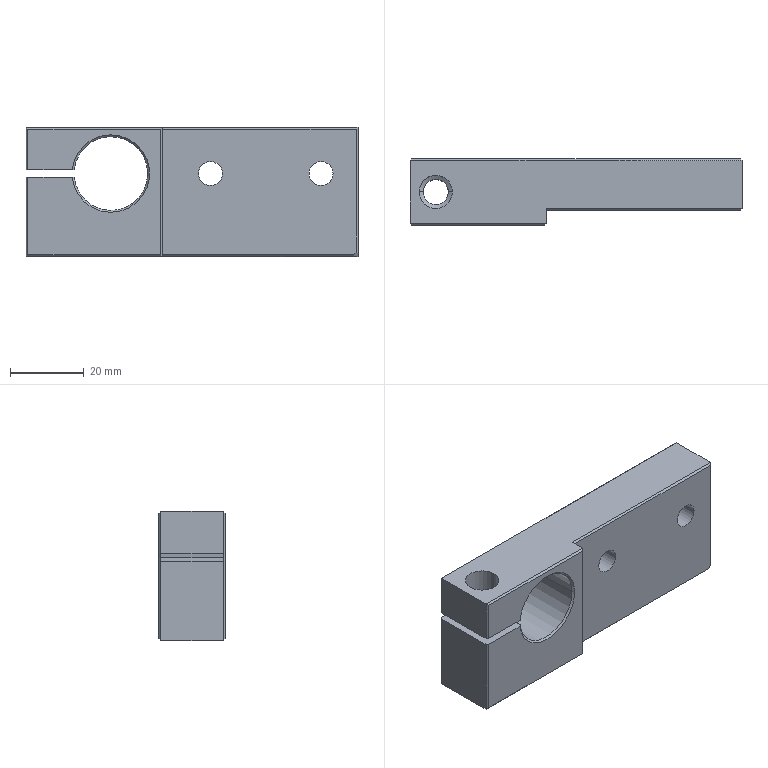Part | NX | 1 solid | 46 faces | box 90 x 18 x 35 mm | volume 39820 mm3 | plane 27 | cylinder 14 | cone 5 | commonest cylinder face diameters 6.5 x4 11 x4 6.8 x2 9 x2 20 x2
STEP:
#1=CARTESIAN_POINT('',(0.5,18.,-17.));
#2=VERTEX_POINT('',#1);
#3=CARTESIAN_POINT('',(0.,17.5,-17.5));
#4=VERTEX_POINT('',#3);
#5=CARTESIAN_POINT('',(17.5,35.,0.));
#6=DIRECTION('',(-0.5774,-0.5774,-0.5774));
#7=VECTOR('',#6,1000.);
#8=LINE('',#5,#7);
#9=EDGE_CURVE('',#2,#4,#8,.T.);
#10=ORIENTED_EDGE('',*,*,#9,.T.);
#11=CARTESIAN_POINT('',(0.,17.5,4.));
#12=VERTEX_POINT('',#11);
#13=CARTESIAN_POINT('',(0.,17.5,0.));
#14=DIRECTION('',(0.,0.,1.));
#15=VECTOR('',#14,1000.);
#16=LINE('',#13,#15);
#17=EDGE_CURVE('',#4,#12,#16,.T.);
#18=ORIENTED_EDGE('',*,*,#17,.T.);
#19=CARTESIAN_POINT('',(0.5,18.,4.));
#20=VERTEX_POINT('',#19);
#21=CARTESIAN_POINT('',(-17.5,0.,4.));
#22=DIRECTION('',(0.7071,0.7071,0.));
#23=VECTOR('',#22,1000.);
#24=LINE('',#21,#23);
#25=EDGE_CURVE('',#12,#20,#24,.T.);
#26=ORIENTED_EDGE('',*,*,#25,.T.);
#27=CARTESIAN_POINT('',(0.5,18.,0.));
#28=DIRECTION('',(0.,0.,1.));
#29=VECTOR('',#28,1000.);
#30=LINE('',#27,#29);
#31=EDGE_CURVE('',#2,#20,#30,.T.);
#32=ORIENTED_EDGE('',*,*,#31,.F.);
#33=EDGE_LOOP('',(#10,#18,#26,#32));
#34=FACE_BOUND('',#33,.T.);
#35=CARTESIAN_POINT('',(0.,17.5,-16.5));
#36=DIRECTION('',(-0.7071,0.7071,0.));
#37=DIRECTION('',(0.,0.,1.));
#38=AXIS2_PLACEMENT_3D('',#35,#36,#37);
#39=PLANE('',#38);
#40=ADVANCED_FACE('',(#34),#39,.T.);
#41=CARTESIAN_POINT('',(37.,0.5,-17.5));
#42=VERTEX_POINT('',#41);
#43=CARTESIAN_POINT('',(36.5,0.,-17.));
#44=VERTEX_POINT('',#43);
#45=CARTESIAN_POINT('',(19.5,-17.,0.));
#46=DIRECTION('',(-0.5774,-0.5774,0.5774));
#47=VECTOR('',#46,1000.);
#48=LINE('',#45,#47);
#49=EDGE_CURVE('',#42,#44,#48,.T.);
#50=ORIENTED_EDGE('',*,*,#49,.T.);
#51=CARTESIAN_POINT('',(0.5,0.,-17.));
#52=VERTEX_POINT('',#51);
#53=CARTESIAN_POINT('',(0.,0.,-17.));
#54=DIRECTION('',(1.,0.,0.));
#55=VECTOR('',#54,1000.);
#56=LINE('',#53,#55);
#57=EDGE_CURVE('',#52,#44,#56,.T.);
#58=ORIENTED_EDGE('',*,*,#57,.F.);
#59=CARTESIAN_POINT('',(0.,0.5,-17.5));
#60=VERTEX_POINT('',#59);
#61=CARTESIAN_POINT('',(17.5,-17.,0.));
#62=DIRECTION('',(0.5774,-0.5774,0.5774));
#63=VECTOR('',#62,1000.);
#64=LINE('',#61,#63);
#65=EDGE_CURVE('',#60,#52,#64,.T.);
#66=ORIENTED_EDGE('',*,*,#65,.F.);
#67=CARTESIAN_POINT('',(0.,0.5,-17.5));
#68=DIRECTION('',(-1.,0.,0.));
#69=VECTOR('',#68,1000.);
#70=LINE('',#67,#69);
#71=EDGE_CURVE('',#42,#60,#70,.T.);
#72=ORIENTED_EDGE('',*,*,#71,.F.);
#73=EDGE_LOOP('',(#50,#58,#66,#72));
#74=FACE_BOUND('',#73,.T.);
#75=CARTESIAN_POINT('',(1.,0.5,-17.5));
#76=DIRECTION('',(0.,-0.7071,-0.7071));
#77=DIRECTION('',(0.,-0.7071,0.7071));
#78=AXIS2_PLACEMENT_3D('',#75,#76,#77);
#79=PLANE('',#78);
#80=ADVANCED_FACE('',(#74),#79,.T.);
#81=CARTESIAN_POINT('',(37.,4.,17.));
#82=VERTEX_POINT('',#81);
#83=CARTESIAN_POINT('',(37.,4.,-17.));
#84=VERTEX_POINT('',#83);
#85=CARTESIAN_POINT('',(37.,4.,0.));
#86=DIRECTION('',(0.,0.,-1.));
#87=VECTOR('',#86,1000.);
#88=LINE('',#85,#87);
#89=EDGE_CURVE('',#82,#84,#88,.T.);
#90=ORIENTED_EDGE('',*,*,#89,.F.);
#91=CARTESIAN_POINT('',(37.,4.5,17.5));
#92=VERTEX_POINT('',#91);
#93=CARTESIAN_POINT('',(37.,-13.,0.));
#94=DIRECTION('',(0.,-0.7071,-0.7071));
#95=VECTOR('',#94,1000.);
#96=LINE('',#93,#95);
#97=EDGE_CURVE('',#92,#82,#96,.T.);
#98=ORIENTED_EDGE('',*,*,#97,.F.);
#99=CARTESIAN_POINT('',(37.,0.5,17.5));
#100=VERTEX_POINT('',#99);
#101=CARTESIAN_POINT('',(37.,0.,17.5));
#102=DIRECTION('',(0.,-1.,0.));
#103=VECTOR('',#102,1000.);
#104=LINE('',#101,#103);
#105=EDGE_CURVE('',#92,#100,#104,.T.);
#106=ORIENTED_EDGE('',*,*,#105,.T.);
#107=CARTESIAN_POINT('',(37.,0.5,0.));
#108=DIRECTION('',(0.,0.,-1.));
#109=VECTOR('',#108,1000.);
#110=LINE('',#107,#109);
#111=EDGE_CURVE('',#100,#42,#110,.T.);
#112=ORIENTED_EDGE('',*,*,#111,.T.);
#113=CARTESIAN_POINT('',(37.,4.5,-17.5));
#114=VERTEX_POINT('',#113);
#115=CARTESIAN_POINT('',(37.,0.,-17.5));
#116=DIRECTION('',(0.,1.,0.));
#117=VECTOR('',#116,1000.);
#118=LINE('',#115,#117);
#119=EDGE_CURVE('',#42,#114,#118,.T.);
#120=ORIENTED_EDGE('',*,*,#119,.T.);
#121=CARTESIAN_POINT('',(37.,-13.,0.));
#122=DIRECTION('',(0.,0.7071,-0.7071));
#123=VECTOR('',#122,1000.);
#124=LINE('',#121,#123);
#125=EDGE_CURVE('',#84,#114,#124,.T.);
#126=ORIENTED_EDGE('',*,*,#125,.F.);
#127=EDGE_LOOP('',(#90,#98,#106,#112,#120,#126));
#128=FACE_BOUND('',#127,.T.);
#129=CARTESIAN_POINT('',(37.,0.,-17.5));
#130=DIRECTION('',(1.,0.,0.));
#131=DIRECTION('',(0.,1.,0.));
#132=AXIS2_PLACEMENT_3D('',#129,#130,#131);
#133=PLANE('',#132);
#134=ADVANCED_FACE('',(#128),#133,.T.);
#135=CARTESIAN_POINT('',(44.5,11.5,5.));
#136=VERTEX_POINT('',#135);
#137=CARTESIAN_POINT('',(55.5,11.5,5.));
#138=VERTEX_POINT('',#137);
#139=CARTESIAN_POINT('',(50.,11.5,5.));
#140=DIRECTION('',(0.,1.,0.));
#141=DIRECTION('',(1.,0.,0.));
#142=AXIS2_PLACEMENT_3D('',#139,#140,#141);
#143=CIRCLE('',#142,5.5);
#144=EDGE_CURVE('',#136,#138,#143,.T.);
#145=ORIENTED_EDGE('',*,*,#144,.T.);
#146=CARTESIAN_POINT('',(50.,11.5,5.));
#147=DIRECTION('',(0.,1.,0.));
#148=DIRECTION('',(1.,0.,0.));
#149=AXIS2_PLACEMENT_3D('',#146,#147,#148);
#150=CIRCLE('',#149,5.5);
#151=EDGE_CURVE('',#138,#136,#150,.T.);
#152=ORIENTED_EDGE('',*,*,#151,.T.);
#153=EDGE_LOOP('',(#145,#152));
#154=FACE_BOUND('',#153,.T.);
#155=CARTESIAN_POINT('',(53.25,11.5,5.));
#156=VERTEX_POINT('',#155);
#157=CARTESIAN_POINT('',(46.75,11.5,5.));
#158=VERTEX_POINT('',#157);
#159=CARTESIAN_POINT('',(50.,11.5,5.));
#160=DIRECTION('',(0.,1.,0.));
#161=DIRECTION('',(1.,0.,0.));
#162=AXIS2_PLACEMENT_3D('',#159,#160,#161);
#163=CIRCLE('',#162,3.25);
#164=EDGE_CURVE('',#156,#158,#163,.T.);
#165=ORIENTED_EDGE('',*,*,#164,.F.);
#166=CARTESIAN_POINT('',(50.,11.5,5.));
#167=DIRECTION('',(0.,1.,0.));
#168=DIRECTION('',(1.,0.,0.));
#169=AXIS2_PLACEMENT_3D('',#166,#167,#168);
#170=CIRCLE('',#169,3.25);
#171=EDGE_CURVE('',#158,#156,#170,.T.);
#172=ORIENTED_EDGE('',*,*,#171,.F.);
#173=EDGE_LOOP('',(#165,#172));
#174=FACE_BOUND('',#173,.T.);
#175=CARTESIAN_POINT('',(50.,11.5,5.));
#176=DIRECTION('',(0.,1.,0.));
#177=DIRECTION('',(1.,0.,0.));
#178=AXIS2_PLACEMENT_3D('',#175,#176,#177);
#179=PLANE('',#178);
#180=ADVANCED_FACE('',(#154,#174),#179,.T.);
#181=CARTESIAN_POINT('',(74.5,11.5,5.));
#182=VERTEX_POINT('',#181);
#183=CARTESIAN_POINT('',(85.5,11.5,5.));
#184=VERTEX_POINT('',#183);
#185=CARTESIAN_POINT('',(80.,11.5,5.));
#186=DIRECTION('',(0.,1.,0.));
#187=DIRECTION('',(1.,0.,0.));
#188=AXIS2_PLACEMENT_3D('',#185,#186,#187);
#189=CIRCLE('',#188,5.5);
#190=EDGE_CURVE('',#182,#184,#189,.T.);
#191=ORIENTED_EDGE('',*,*,#190,.F.);
#192=CARTESIAN_POINT('',(74.5,18.,5.));
#193=VERTEX_POINT('',#192);
#194=CARTESIAN_POINT('',(74.5,-2.79,5.));
#195=DIRECTION('',(0.,1.,0.));
#196=VECTOR('',#195,1000.);
#197=LINE('',#194,#196);
#198=EDGE_CURVE('',#182,#193,#197,.T.);
#199=ORIENTED_EDGE('',*,*,#198,.T.);
#200=CARTESIAN_POINT('',(85.5,18.,5.));
#201=VERTEX_POINT('',#200);
#202=CARTESIAN_POINT('',(80.,18.,5.));
#203=DIRECTION('',(0.,1.,0.));
#204=DIRECTION('',(1.,0.,0.));
#205=AXIS2_PLACEMENT_3D('',#202,#203,#204);
#206=CIRCLE('',#205,5.5);
#207=EDGE_CURVE('',#193,#201,#206,.T.);
#208=ORIENTED_EDGE('',*,*,#207,.T.);
#209=CARTESIAN_POINT('',(85.5,-2.79,5.));
#210=DIRECTION('',(0.,1.,0.));
#211=VECTOR('',#210,1000.);
#212=LINE('',#209,#211);
#213=EDGE_CURVE('',#184,#201,#212,.T.);
#214=ORIENTED_EDGE('',*,*,#213,.F.);
#215=EDGE_LOOP('',(#191,#199,#208,#214));
#216=FACE_BOUND('',#215,.T.);
#217=CARTESIAN_POINT('',(80.,-2.79,5.));
#218=DIRECTION('',(0.,1.,0.));
#219=DIRECTION('',(1.,0.,0.));
#220=AXIS2_PLACEMENT_3D('',#217,#218,#219);
#221=CYLINDRICAL_SURFACE('',#220,5.5);
#222=ADVANCED_FACE('',(#216),#221,.F.);
#223=CARTESIAN_POINT('',(90.,17.5,17.5));
#224=VERTEX_POINT('',#223);
#225=CARTESIAN_POINT('',(89.5,18.,17.));
#226=VERTEX_POINT('',#225);
#227=CARTESIAN_POINT('',(72.5,35.,0.));
#228=DIRECTION('',(-0.5774,0.5774,-0.5774));
#229=VECTOR('',#228,1000.);
#230=LINE('',#227,#229);
#231=EDGE_CURVE('',#224,#226,#230,.T.);
#232=ORIENTED_EDGE('',*,*,#231,.F.);
#233=CARTESIAN_POINT('',(90.,17.5,-17.5));
#234=VERTEX_POINT('',#233);
#235=CARTESIAN_POINT('',(90.,17.5,0.));
#236=DIRECTION('',(0.,0.,-1.));
#237=VECTOR('',#236,1000.);
#238=LINE('',#235,#237);
#239=EDGE_CURVE('',#224,#234,#238,.T.);
#240=ORIENTED_EDGE('',*,*,#239,.T.);
#241=CARTESIAN_POINT('',(89.5,18.,-17.));
#242=VERTEX_POINT('',#241);
#243=CARTESIAN_POINT('',(72.5,35.,0.));
#244=DIRECTION('',(-0.5774,0.5774,0.5774));
#245=VECTOR('',#244,1000.);
#246=LINE('',#243,#245);
#247=EDGE_CURVE('',#234,#242,#246,.T.);
#248=ORIENTED_EDGE('',*,*,#247,.T.);
#249=CARTESIAN_POINT('',(89.5,18.,0.));
#250=DIRECTION('',(0.,0.,1.));
#251=VECTOR('',#250,1000.);
#252=LINE('',#249,#251);
#253=EDGE_CURVE('',#242,#226,#252,.T.);
#254=ORIENTED_EDGE('',*,*,#253,.T.);
#255=EDGE_LOOP('',(#232,#240,#248,#254));
#256=FACE_BOUND('',#255,.T.);
#257=CARTESIAN_POINT('',(89.5,18.,-16.5));
#258=DIRECTION('',(0.7071,0.7071,0.));
#259=DIRECTION('',(0.,0.,-1.));
#260=AXIS2_PLACEMENT_3D('',#257,#258,#259);
#261=PLANE('',#260);
#262=ADVANCED_FACE('',(#256),#261,.T.);
#263=CARTESIAN_POINT('',(10.4,9.,-17.5));
#264=VERTEX_POINT('',#263);
#265=CARTESIAN_POINT('',(3.6,9.,-17.5));
#266=VERTEX_POINT('',#265);
#267=CARTESIAN_POINT('',(7.,9.,-17.5));
#268=DIRECTION('',(0.,0.,1.));
#269=DIRECTION('',(1.,0.,0.));
#270=AXIS2_PLACEMENT_3D('',#267,#268,#269);
#271=CIRCLE('',#270,3.4);
#272=EDGE_CURVE('',#264,#266,#271,.T.);
#273=ORIENTED_EDGE('',*,*,#272,.F.);
#274=CARTESIAN_POINT('',(10.4,9.,3.329));
#275=VERTEX_POINT('',#274);
#276=CARTESIAN_POINT('',(10.4,9.,4.));
#277=DIRECTION('',(0.,0.,1.));
#278=VECTOR('',#277,1000.);
#279=LINE('',#276,#278);
#280=EDGE_CURVE('',#264,#275,#279,.T.);
#281=ORIENTED_EDGE('',*,*,#280,.T.);
#282=CARTESIAN_POINT('',(3.6,9.,3.329));
#283=VERTEX_POINT('',#282);
#284=CARTESIAN_POINT('',(7.,9.,3.329));
#285=DIRECTION('',(0.,0.,1.));
#286=DIRECTION('',(1.,0.,0.));
#287=AXIS2_PLACEMENT_3D('',#284,#285,#286);
#288=CIRCLE('',#287,3.4);
#289=EDGE_CURVE('',#275,#283,#288,.T.);
#290=ORIENTED_EDGE('',*,*,#289,.T.);
#291=CARTESIAN_POINT('',(3.6,9.,4.));
#292=DIRECTION('',(0.,0.,1.));
#293=VECTOR('',#292,1000.);
#294=LINE('',#291,#293);
#295=EDGE_CURVE('',#266,#283,#294,.T.);
#296=ORIENTED_EDGE('',*,*,#295,.F.);
#297=EDGE_LOOP('',(#273,#281,#290,#296));
#298=FACE_BOUND('',#297,.T.);
#299=CARTESIAN_POINT('',(7.,9.,4.));
#300=DIRECTION('',(0.,0.,1.));
#301=DIRECTION('',(1.,0.,0.));
#302=AXIS2_PLACEMENT_3D('',#299,#300,#301);
#303=CYLINDRICAL_SURFACE('',#302,3.4);
#304=ADVANCED_FACE('',(#298),#303,.F.);
#305=CARTESIAN_POINT('',(76.75,4.,5.));
#306=VERTEX_POINT('',#305);
#307=CARTESIAN_POINT('',(83.25,4.,5.));
#308=VERTEX_POINT('',#307);
#309=CARTESIAN_POINT('',(80.,4.,5.));
#310=DIRECTION('',(0.,1.,0.));
#311=DIRECTION('',(1.,0.,0.));
#312=AXIS2_PLACEMENT_3D('',#309,#310,#311);
#313=CIRCLE('',#312,3.25);
#314=EDGE_CURVE('',#306,#308,#313,.T.);
#315=ORIENTED_EDGE('',*,*,#314,.F.);
#316=CARTESIAN_POINT('',(76.75,11.5,5.));
#317=VERTEX_POINT('',#316);
#318=CARTESIAN_POINT('',(76.75,-2.79,5.));
#319=DIRECTION('',(0.,1.,0.));
#320=VECTOR('',#319,1000.);
#321=LINE('',#318,#320);
#322=EDGE_CURVE('',#306,#317,#321,.T.);
#323=ORIENTED_EDGE('',*,*,#322,.T.);
#324=CARTESIAN_POINT('',(83.25,11.5,5.));
#325=VERTEX_POINT('',#324);
#326=CARTESIAN_POINT('',(80.,11.5,5.));
#327=DIRECTION('',(0.,1.,0.));
#328=DIRECTION('',(1.,0.,0.));
#329=AXIS2_PLACEMENT_3D('',#326,#327,#328);
#330=CIRCLE('',#329,3.25);
#331=EDGE_CURVE('',#317,#325,#330,.T.);
#332=ORIENTED_EDGE('',*,*,#331,.T.);
#333=CARTESIAN_POINT('',(83.25,-2.79,5.));
#334=DIRECTION('',(0.,1.,0.));
#335=VECTOR('',#334,1000.);
#336=LINE('',#333,#335);
#337=EDGE_CURVE('',#308,#325,#336,.T.);
#338=ORIENTED_EDGE('',*,*,#337,.F.);
#339=EDGE_LOOP('',(#315,#323,#332,#338));
#340=FACE_BOUND('',#339,.T.);
#341=CARTESIAN_POINT('',(80.,-2.79,5.));
#342=DIRECTION('',(0.,1.,0.));
#343=DIRECTION('',(1.,0.,0.));
#344=AXIS2_PLACEMENT_3D('',#341,#342,#343);
#345=CYLINDRICAL_SURFACE('',#344,3.25);
#346=ADVANCED_FACE('',(#340),#345,.F.);
#347=CARTESIAN_POINT('',(90.,5.207,-17.5));
#348=VERTEX_POINT('',#347);
#349=CARTESIAN_POINT('',(90.,4.5,-16.5));
#350=VERTEX_POINT('',#349);
#351=CARTESIAN_POINT('',(90.,-7.167,0.));
#352=DIRECTION('',(0.,-0.5774,0.8165));
#353=VECTOR('',#352,1000.);
#354=LINE('',#351,#353);
#355=EDGE_CURVE('',#348,#350,#354,.T.);
#356=ORIENTED_EDGE('',*,*,#355,.T.);
#357=CARTESIAN_POINT('',(89.5,4.,-16.293));
#358=VERTEX_POINT('',#357);
#359=CARTESIAN_POINT('',(0.,-85.5,20.779));
#360=DIRECTION('',(-0.6786,-0.6786,0.2811));
#361=VECTOR('',#360,1000.);
#362=LINE('',#359,#361);
#363=EDGE_CURVE('',#350,#358,#362,.T.);
#364=ORIENTED_EDGE('',*,*,#363,.T.);
#365=CARTESIAN_POINT('',(88.793,4.,-17.));
#366=VERTEX_POINT('',#365);
#367=CARTESIAN_POINT('',(105.793,4.,0.));
#368=DIRECTION('',(-0.7071,0.,-0.7071));
#369=VECTOR('',#368,1000.);
#370=LINE('',#367,#369);
#371=EDGE_CURVE('',#358,#366,#370,.T.);
#372=ORIENTED_EDGE('',*,*,#371,.T.);
#373=CARTESIAN_POINT('',(89.,4.5,-17.5));
#374=VERTEX_POINT('',#373);
#375=CARTESIAN_POINT('',(81.751,-13.,0.));
#376=DIRECTION('',(0.2811,0.6786,-0.6786));
#377=VECTOR('',#376,1000.);
#378=LINE('',#375,#377);
#379=EDGE_CURVE('',#366,#374,#378,.T.);
#380=ORIENTED_EDGE('',*,*,#379,.T.);
#381=CARTESIAN_POINT('',(0.,-58.433,-17.5));
#382=DIRECTION('',(-0.8165,-0.5774,0.));
#383=VECTOR('',#382,1000.);
#384=LINE('',#381,#383);
#385=EDGE_CURVE('',#348,#374,#384,.T.);
#386=ORIENTED_EDGE('',*,*,#385,.F.);
#387=EDGE_LOOP('',(#356,#364,#372,#380,#386));
#388=FACE_BOUND('',#387,.T.);
#389=CARTESIAN_POINT('',(89.,4.5,-17.5));
#390=DIRECTION('',(0.5,-0.7071,-0.5));
#391=DIRECTION('',(0.,0.5774,-0.8165));
#392=AXIS2_PLACEMENT_3D('',#389,#390,#391);
#393=PLANE('',#392);
#394=ADVANCED_FACE('',(#388),#393,.T.);
#395=CARTESIAN_POINT('',(0.,4.5,-17.5));
#396=DIRECTION('',(1.,0.,0.));
#397=VECTOR('',#396,1000.);
#398=LINE('',#395,#397);
#399=EDGE_CURVE('',#114,#374,#398,.T.);
#400=ORIENTED_EDGE('',*,*,#399,.T.);
#401=ORIENTED_EDGE('',*,*,#379,.F.);
#402=CARTESIAN_POINT('',(0.,4.,-17.));
#403=DIRECTION('',(-1.,0.,0.));
#404=VECTOR('',#403,1000.);
#405=LINE('',#402,#404);
#406=EDGE_CURVE('',#366,#84,#405,.T.);
#407=ORIENTED_EDGE('',*,*,#406,.T.);
#408=ORIENTED_EDGE('',*,*,#125,.T.);
#409=EDGE_LOOP('',(#400,#401,#407,#408));
#410=FACE_BOUND('',#409,.T.);
#411=CARTESIAN_POINT('',(37.,4.5,-17.5));
#412=DIRECTION('',(0.,-0.7071,-0.7071));
#413=DIRECTION('',(0.,-0.7071,0.7071));
#414=AXIS2_PLACEMENT_3D('',#411,#412,#413);
#415=PLANE('',#414);
#416=ADVANCED_FACE('',(#410),#415,.T.);
#417=CARTESIAN_POINT('',(0.,0.5,17.5));
#418=VERTEX_POINT('',#417);
#419=CARTESIAN_POINT('',(0.5,0.,17.));
#420=VERTEX_POINT('',#419);
#421=CARTESIAN_POINT('',(17.5,-17.,0.));
#422=DIRECTION('',(0.5774,-0.5774,-0.5774));
#423=VECTOR('',#422,1000.);
#424=LINE('',#421,#423);
#425=EDGE_CURVE('',#418,#420,#424,.T.);
#426=ORIENTED_EDGE('',*,*,#425,.F.);
#427=CARTESIAN_POINT('',(0.,0.5,6.));
#428=VERTEX_POINT('',#427);
#429=CARTESIAN_POINT('',(0.,0.5,0.));
#430=DIRECTION('',(0.,0.,1.));
#431=VECTOR('',#430,1000.);
#432=LINE('',#429,#431);
#433=EDGE_CURVE('',#428,#418,#432,.T.);
#434=ORIENTED_EDGE('',*,*,#433,.F.);
#435=CARTESIAN_POINT('',(0.5,0.,6.));
#436=VERTEX_POINT('',#435);
#437=CARTESIAN_POINT('',(0.5,0.,6.));
#438=DIRECTION('',(0.7071,-0.7071,0.));
#439=VECTOR('',#438,1000.);
#440=LINE('',#437,#439);
#441=EDGE_CURVE('',#428,#436,#440,.T.);
#442=ORIENTED_EDGE('',*,*,#441,.T.);
#443=CARTESIAN_POINT('',(0.5,0.,0.));
#444=DIRECTION('',(0.,0.,-1.));
#445=VECTOR('',#444,1000.);
#446=LINE('',#443,#445);
#447=EDGE_CURVE('',#420,#436,#446,.T.);
#448=ORIENTED_EDGE('',*,*,#447,.F.);
#449=EDGE_LOOP('',(#426,#434,#442,#448));
#450=FACE_BOUND('',#449,.T.);
#451=CARTESIAN_POINT('',(0.5,0.,6.));
#452=DIRECTION('',(-0.7071,-0.7071,0.));
#453=DIRECTION('',(-0.7071,0.7071,0.));
#454=AXIS2_PLACEMENT_3D('',#451,#452,#453);
#455=PLANE('',#454);
#456=ADVANCED_FACE('',(#450),#455,.T.);
#457=ORIENTED_EDGE('',*,*,#111,.F.);
#458=CARTESIAN_POINT('',(36.5,0.,17.));
#459=VERTEX_POINT('',#458);
#460=CARTESIAN_POINT('',(19.5,-17.,0.));
#461=DIRECTION('',(-0.5774,-0.5774,-0.5774));
#462=VECTOR('',#461,1000.);
#463=LINE('',#460,#462);
#464=EDGE_CURVE('',#100,#459,#463,.T.);
#465=ORIENTED_EDGE('',*,*,#464,.T.);
#466=CARTESIAN_POINT('',(36.5,0.,0.));
#467=DIRECTION('',(0.,0.,1.));
#468=VECTOR('',#467,1000.);
#469=LINE('',#466,#468);
#470=EDGE_CURVE('',#44,#459,#469,.T.);
#471=ORIENTED_EDGE('',*,*,#470,.F.);
#472=ORIENTED_EDGE('',*,*,#49,.F.);
#473=EDGE_LOOP('',(#457,#465,#471,#472));
#474=FACE_BOUND('',#473,.T.);
#475=CARTESIAN_POINT('',(37.,0.5,-17.));
#476=DIRECTION('',(0.7071,-0.7071,0.));
#477=DIRECTION('',(0.,0.,-1.));
#478=AXIS2_PLACEMENT_3D('',#475,#476,#477);
#479=PLANE('',#478);
#480=ADVANCED_FACE('',(#474),#479,.T.);
#481=ORIENTED_EDGE('',*,*,#119,.F.);
#482=ORIENTED_EDGE('',*,*,#71,.T.);
#483=CARTESIAN_POINT('',(0.,0.,-17.5));
#484=DIRECTION('',(0.,1.,0.));
#485=VECTOR('',#484,1000.);
#486=LINE('',#483,#485);
#487=EDGE_CURVE('',#60,#4,#486,.T.);
#488=ORIENTED_EDGE('',*,*,#487,.T.);
#489=CARTESIAN_POINT('',(0.,17.5,-17.5));
#490=DIRECTION('',(1.,0.,0.));
#491=VECTOR('',#490,1000.);
#492=LINE('',#489,#491);
#493=EDGE_CURVE('',#4,#234,#492,.T.);
#494=ORIENTED_EDGE('',*,*,#493,.T.);
#495=CARTESIAN_POINT('',(90.,0.,-17.5));
#496=DIRECTION('',(0.,-1.,0.));
#497=VECTOR('',#496,1000.);
#498=LINE('',#495,#497);
#499=EDGE_CURVE('',#234,#348,#498,.T.);
#500=ORIENTED_EDGE('',*,*,#499,.T.);
#501=ORIENTED_EDGE('',*,*,#385,.T.);
#502=ORIENTED_EDGE('',*,*,#399,.F.);
#503=EDGE_LOOP('',(#481,#482,#488,#494,#500,#501,#502));
#504=FACE_BOUND('',#503,.T.);
#505=ORIENTED_EDGE('',*,*,#272,.T.);
#506=CARTESIAN_POINT('',(7.,9.,-17.5));
#507=DIRECTION('',(0.,0.,1.));
#508=DIRECTION('',(1.,0.,0.));
#509=AXIS2_PLACEMENT_3D('',#506,#507,#508);
#510=CIRCLE('',#509,3.4);
#511=EDGE_CURVE('',#266,#264,#510,.T.);
#512=ORIENTED_EDGE('',*,*,#511,.T.);
#513=EDGE_LOOP('',(#505,#512));
#514=FACE_BOUND('',#513,.T.);
#515=CARTESIAN_POINT('',(0.,0.,-17.5));
#516=DIRECTION('',(0.,0.,1.));
#517=DIRECTION('',(1.,0.,0.));
#518=AXIS2_PLACEMENT_3D('',#515,#516,#517);
#519=PLANE('',#518);
#520=ADVANCED_FACE('',(#504,#514),#519,.F.);
#521=CARTESIAN_POINT('',(90.,4.5,17.5));
#522=VERTEX_POINT('',#521);
#523=CARTESIAN_POINT('',(90.,0.,17.5));
#524=DIRECTION('',(0.,-1.,0.));
#525=VECTOR('',#524,1000.);
#526=LINE('',#523,#525);
#527=EDGE_CURVE('',#224,#522,#526,.T.);
#528=ORIENTED_EDGE('',*,*,#527,.F.);
#529=CARTESIAN_POINT('',(0.,17.5,17.5));
#530=VERTEX_POINT('',#529);
#531=CARTESIAN_POINT('',(0.,17.5,17.5));
#532=DIRECTION('',(-1.,0.,0.));
#533=VECTOR('',#532,1000.);
#534=LINE('',#531,#533);
#535=EDGE_CURVE('',#224,#530,#534,.T.);
#536=ORIENTED_EDGE('',*,*,#535,.T.);
#537=CARTESIAN_POINT('',(0.,0.,17.5));
#538=DIRECTION('',(0.,1.,0.));
#539=VECTOR('',#538,1000.);
#540=LINE('',#537,#539);
#541=EDGE_CURVE('',#418,#530,#540,.T.);
#542=ORIENTED_EDGE('',*,*,#541,.F.);
#543=CARTESIAN_POINT('',(0.,0.5,17.5));
#544=DIRECTION('',(1.,0.,0.));
#545=VECTOR('',#544,1000.);
#546=LINE('',#543,#545);
#547=EDGE_CURVE('',#418,#100,#546,.T.);
#548=ORIENTED_EDGE('',*,*,#547,.T.);
#549=ORIENTED_EDGE('',*,*,#105,.F.);
#550=CARTESIAN_POINT('',(0.,4.5,17.5));
#551=DIRECTION('',(1.,0.,0.));
#552=VECTOR('',#551,1000.);
#553=LINE('',#550,#552);
#554=EDGE_CURVE('',#92,#522,#553,.T.);
#555=ORIENTED_EDGE('',*,*,#554,.T.);
#556=EDGE_LOOP('',(#528,#536,#542,#548,#549,#555));
#557=FACE_BOUND('',#556,.T.);
#558=CARTESIAN_POINT('',(11.5,9.,17.5));
#559=VERTEX_POINT('',#558);
#560=CARTESIAN_POINT('',(2.5,9.,17.5));
#561=VERTEX_POINT('',#560);
#562=CARTESIAN_POINT('',(7.,9.,17.5));
#563=DIRECTION('',(0.,0.,-1.));
#564=DIRECTION('',(-1.,0.,0.));
#565=AXIS2_PLACEMENT_3D('',#562,#563,#564);
#566=CIRCLE('',#565,4.5);
#567=EDGE_CURVE('',#559,#561,#566,.T.);
#568=ORIENTED_EDGE('',*,*,#567,.T.);
#569=CARTESIAN_POINT('',(7.,9.,17.5));
#570=DIRECTION('',(0.,0.,-1.));
#571=DIRECTION('',(-1.,0.,0.));
#572=AXIS2_PLACEMENT_3D('',#569,#570,#571);
#573=CIRCLE('',#572,4.5);
#574=EDGE_CURVE('',#561,#559,#573,.T.);
#575=ORIENTED_EDGE('',*,*,#574,.T.);
#576=EDGE_LOOP('',(#568,#575));
#577=FACE_BOUND('',#576,.T.);
#578=CARTESIAN_POINT('',(0.,0.,17.5));
#579=DIRECTION('',(0.,0.,1.));
#580=DIRECTION('',(1.,0.,0.));
#581=AXIS2_PLACEMENT_3D('',#578,#579,#580);
#582=PLANE('',#581);
#583=ADVANCED_FACE('',(#557,#577),#582,.T.);
#584=CARTESIAN_POINT('',(12.548,0.,6.));
#585=VERTEX_POINT('',#584);
#586=CARTESIAN_POINT('',(0.,0.,6.));
#587=DIRECTION('',(1.,0.,0.));
#588=VECTOR('',#587,1000.);
#589=LINE('',#586,#588);
#590=EDGE_CURVE('',#436,#585,#589,.T.);
#591=ORIENTED_EDGE('',*,*,#590,.F.);
#592=ORIENTED_EDGE('',*,*,#441,.F.);
#593=CARTESIAN_POINT('',(0.,17.5,6.));
#594=VERTEX_POINT('',#593);
#595=CARTESIAN_POINT('',(0.,0.,6.));
#596=DIRECTION('',(0.,-1.,0.));
#597=VECTOR('',#596,1000.);
#598=LINE('',#595,#597);
#599=EDGE_CURVE('',#594,#428,#598,.T.);
#600=ORIENTED_EDGE('',*,*,#599,.F.);
#601=CARTESIAN_POINT('',(0.5,18.,6.));
#602=VERTEX_POINT('',#601);
#603=CARTESIAN_POINT('',(-17.5,0.,6.));
#604=DIRECTION('',(-0.7071,-0.7071,0.));
#605=VECTOR('',#604,1000.);
#606=LINE('',#603,#605);
#607=EDGE_CURVE('',#602,#594,#606,.T.);
#608=ORIENTED_EDGE('',*,*,#607,.F.);
#609=CARTESIAN_POINT('',(12.548,18.,6.));
#610=VERTEX_POINT('',#609);
#611=CARTESIAN_POINT('',(0.,18.,6.));
#612=DIRECTION('',(-1.,0.,0.));
#613=VECTOR('',#612,1000.);
#614=LINE('',#611,#613);
#615=EDGE_CURVE('',#610,#602,#614,.T.);
#616=ORIENTED_EDGE('',*,*,#615,.F.);
#617=CARTESIAN_POINT('',(13.05,17.5,6.));
#618=VERTEX_POINT('',#617);
#619=CARTESIAN_POINT('',(12.548,18.,6.));
#620=CARTESIAN_POINT('',(12.604,17.944,6.));
#621=CARTESIAN_POINT('',(12.715,17.833,6.));
#622=CARTESIAN_POINT('',(12.883,17.667,6.));
#623=CARTESIAN_POINT('',(12.994,17.556,6.));
#624=CARTESIAN_POINT('',(13.05,17.5,6.));
#625=B_SPLINE_CURVE_WITH_KNOTS('',3,(#619,#620,#621,#622,#623,#624),.UNSPECIFIED.,.F.,.F.,(4,1,1,4),(0.,0.3333,0.6667,1.),.UNSPECIFIED.);
#626=EDGE_CURVE('',#610,#618,#625,.T.);
#627=ORIENTED_EDGE('',*,*,#626,.T.);
#628=CARTESIAN_POINT('',(13.05,0.5,6.));
#629=VERTEX_POINT('',#628);
#630=CARTESIAN_POINT('',(13.05,17.5,6.));
#631=DIRECTION('',(0.,-1.,0.));
#632=VECTOR('',#631,1000.);
#633=LINE('',#630,#632);
#634=EDGE_CURVE('',#618,#629,#633,.T.);
#635=ORIENTED_EDGE('',*,*,#634,.T.);
#636=CARTESIAN_POINT('',(13.05,0.5,6.));
#637=CARTESIAN_POINT('',(12.994,0.4444,6.));
#638=CARTESIAN_POINT('',(12.883,0.3333,6.));
#639=CARTESIAN_POINT('',(12.715,0.1667,6.));
#640=CARTESIAN_POINT('',(12.604,0.05556,6.));
#641=CARTESIAN_POINT('',(12.548,0.,6.));
#642=B_SPLINE_CURVE_WITH_KNOTS('',3,(#636,#637,#638,#639,#640,#641),.UNSPECIFIED.,.F.,.F.,(4,1,1,4),(0.,0.3333,0.6667,1.),.UNSPECIFIED.);
#643=EDGE_CURVE('',#629,#585,#642,.T.);
#644=ORIENTED_EDGE('',*,*,#643,.T.);
#645=EDGE_LOOP('',(#591,#592,#600,#608,#616,#627,#635,#644));
#646=FACE_BOUND('',#645,.T.);
#647=CARTESIAN_POINT('',(2.5,9.,6.));
#648=VERTEX_POINT('',#647);
#649=CARTESIAN_POINT('',(11.5,9.,6.));
#650=VERTEX_POINT('',#649);
#651=CARTESIAN_POINT('',(7.,9.,6.));
#652=DIRECTION('',(0.,0.,-1.));
#653=DIRECTION('',(1.,0.,0.));
#654=AXIS2_PLACEMENT_3D('',#651,#652,#653);
#655=CIRCLE('',#654,4.5);
#656=EDGE_CURVE('',#648,#650,#655,.T.);
#657=ORIENTED_EDGE('',*,*,#656,.F.);
#658=CARTESIAN_POINT('',(7.,9.,6.));
#659=DIRECTION('',(0.,0.,-1.));
#660=DIRECTION('',(1.,0.,0.));
#661=AXIS2_PLACEMENT_3D('',#658,#659,#660);
#662=CIRCLE('',#661,4.5);
#663=EDGE_CURVE('',#650,#648,#662,.T.);
#664=ORIENTED_EDGE('',*,*,#663,.F.);
#665=EDGE_LOOP('',(#657,#664));
#666=FACE_BOUND('',#665,.T.);
#667=CARTESIAN_POINT('',(0.,18.,6.));
#668=DIRECTION('',(0.,0.,1.));
#669=DIRECTION('',(1.,0.,0.));
#670=AXIS2_PLACEMENT_3D('',#667,#668,#669);
#671=PLANE('',#670);
#672=ADVANCED_FACE('',(#646,#666),#671,.F.);
#673=ORIENTED_EDGE('',*,*,#547,.F.);
#674=ORIENTED_EDGE('',*,*,#425,.T.);
#675=CARTESIAN_POINT('',(0.,0.,17.));
#676=DIRECTION('',(1.,0.,0.));
#677=VECTOR('',#676,1000.);
#678=LINE('',#675,#677);
#679=EDGE_CURVE('',#420,#459,#678,.T.);
#680=ORIENTED_EDGE('',*,*,#679,.T.);
#681=ORIENTED_EDGE('',*,*,#464,.F.);
#682=EDGE_LOOP('',(#673,#674,#680,#681));
#683=FACE_BOUND('',#682,.T.);
#684=CARTESIAN_POINT('',(1.,0.5,17.5));
#685=DIRECTION('',(0.,0.7071,-0.7071));
#686=DIRECTION('',(-1.,0.,0.));
#687=AXIS2_PLACEMENT_3D('',#684,#685,#686);
#688=PLANE('',#687);
#689=ADVANCED_FACE('',(#683),#688,.F.);
#690=ORIENTED_EDGE('',*,*,#447,.T.);
#691=ORIENTED_EDGE('',*,*,#590,.T.);
#692=CARTESIAN_POINT('',(12.548,0.,4.));
#693=VERTEX_POINT('',#692);
#694=CARTESIAN_POINT('',(23.,0.,5.));
#695=DIRECTION('',(0.,-1.,0.));
#696=DIRECTION('',(-1.,0.,0.));
#697=AXIS2_PLACEMENT_3D('',#694,#695,#696);
#698=CIRCLE('',#697,10.5);
#699=EDGE_CURVE('',#693,#585,#698,.T.);
#700=ORIENTED_EDGE('',*,*,#699,.F.);
#701=CARTESIAN_POINT('',(0.5,0.,4.));
#702=VERTEX_POINT('',#701);
#703=CARTESIAN_POINT('',(0.,0.,4.));
#704=DIRECTION('',(-1.,0.,0.));
#705=VECTOR('',#704,1000.);
#706=LINE('',#703,#705);
#707=EDGE_CURVE('',#693,#702,#706,.T.);
#708=ORIENTED_EDGE('',*,*,#707,.T.);
#709=CARTESIAN_POINT('',(0.5,0.,0.));
#710=DIRECTION('',(0.,0.,1.));
#711=VECTOR('',#710,1000.);
#712=LINE('',#709,#711);
#713=EDGE_CURVE('',#52,#702,#712,.T.);
#714=ORIENTED_EDGE('',*,*,#713,.F.);
#715=ORIENTED_EDGE('',*,*,#57,.T.);
#716=ORIENTED_EDGE('',*,*,#470,.T.);
#717=ORIENTED_EDGE('',*,*,#679,.F.);
#718=EDGE_LOOP('',(#690,#691,#700,#708,#714,#715,#716,#717));
#719=FACE_BOUND('',#718,.T.);
#720=CARTESIAN_POINT('',(0.,0.,-17.5));
#721=DIRECTION('',(0.,-1.,0.));
#722=DIRECTION('',(0.,0.,-1.));
#723=AXIS2_PLACEMENT_3D('',#720,#721,#722);
#724=PLANE('',#723);
#725=ADVANCED_FACE('',(#719),#724,.T.);
#726=ORIENTED_EDGE('',*,*,#567,.F.);
#727=CARTESIAN_POINT('',(11.5,9.,17.5));
#728=DIRECTION('',(0.,0.,-1.));
#729=VECTOR('',#728,1000.);
#730=LINE('',#727,#729);
#731=EDGE_CURVE('',#559,#650,#730,.T.);
#732=ORIENTED_EDGE('',*,*,#731,.T.);
#733=ORIENTED_EDGE('',*,*,#663,.T.);
#734=CARTESIAN_POINT('',(2.5,9.,17.5));
#735=DIRECTION('',(0.,0.,-1.));
#736=VECTOR('',#735,1000.);
#737=LINE('',#734,#736);
#738=EDGE_CURVE('',#561,#648,#737,.T.);
#739=ORIENTED_EDGE('',*,*,#738,.F.);
#740=EDGE_LOOP('',(#726,#732,#733,#739));
#741=FACE_BOUND('',#740,.T.);
#742=CARTESIAN_POINT('',(7.,9.,17.5));
#743=DIRECTION('',(0.,0.,-1.));
#744=DIRECTION('',(-1.,0.,0.));
#745=AXIS2_PLACEMENT_3D('',#742,#743,#744);
#746=CYLINDRICAL_SURFACE('',#745,4.5);
#747=ADVANCED_FACE('',(#741),#746,.F.);
#748=ORIENTED_EDGE('',*,*,#699,.T.);
#749=ORIENTED_EDGE('',*,*,#643,.F.);
#750=CARTESIAN_POINT('',(33.,0.5,5.));
#751=VERTEX_POINT('',#750);
#752=CARTESIAN_POINT('',(23.,0.5,5.));
#753=DIRECTION('',(0.,-1.,0.));
#754=DIRECTION('',(1.,0.,0.));
#755=AXIS2_PLACEMENT_3D('',#752,#753,#754);
#756=CIRCLE('',#755,10.);
#757=EDGE_CURVE('',#751,#629,#756,.T.);
#758=ORIENTED_EDGE('',*,*,#757,.F.);
#759=CARTESIAN_POINT('',(13.05,0.5,4.));
#760=VERTEX_POINT('',#759);
#761=CARTESIAN_POINT('',(23.,0.5,5.));
#762=DIRECTION('',(0.,-1.,0.));
#763=DIRECTION('',(1.,0.,0.));
#764=AXIS2_PLACEMENT_3D('',#761,#762,#763);
#765=CIRCLE('',#764,10.);
#766=EDGE_CURVE('',#760,#751,#765,.T.);
#767=ORIENTED_EDGE('',*,*,#766,.F.);
#768=CARTESIAN_POINT('',(13.05,0.5,4.));
#769=CARTESIAN_POINT('',(13.008,0.4583,4.));
#770=CARTESIAN_POINT('',(12.966,0.4167,4.));
#771=CARTESIAN_POINT('',(12.925,0.375,4.));
#772=CARTESIAN_POINT('',(12.883,0.3333,4.));
#773=CARTESIAN_POINT('',(12.841,0.2917,4.));
#774=CARTESIAN_POINT('',(12.799,0.25,4.));
#775=CARTESIAN_POINT('',(12.757,0.2083,4.));
#776=CARTESIAN_POINT('',(12.715,0.1667,4.));
#777=CARTESIAN_POINT('',(12.673,0.125,4.));
#778=CARTESIAN_POINT('',(12.631,0.08334,4.));
#779=CARTESIAN_POINT('',(12.59,0.04167,4.));
#780=CARTESIAN_POINT('',(12.548,0.,4.));
#781=B_SPLINE_CURVE_WITH_KNOTS('',3,(#768,#769,#770,#771,#772,#773,#774,#775,#776,#777,#778,#779,#780),.UNSPECIFIED.,.F.,.F.,(4,3,3,3,4),(0.,0.1772,0.3544,0.5316,0.7088),.UNSPECIFIED.);
#782=EDGE_CURVE('',#760,#693,#781,.T.);
#783=ORIENTED_EDGE('',*,*,#782,.T.);
#784=EDGE_LOOP('',(#748,#749,#758,#767,#783));
#785=FACE_BOUND('',#784,.T.);
#786=CARTESIAN_POINT('',(23.,0.25,5.));
#787=DIRECTION('',(0.,-1.,0.));
#788=DIRECTION('',(-1.,0.,0.));
#789=AXIS2_PLACEMENT_3D('',#786,#787,#788);
#790=CONICAL_SURFACE('',#789,10.25,0.7854);
#791=ADVANCED_FACE('',(#785),#790,.F.);
#792=CARTESIAN_POINT('',(90.,4.5,0.));
#793=DIRECTION('',(0.,0.,-1.));
#794=VECTOR('',#793,1000.);
#795=LINE('',#792,#794);
#796=EDGE_CURVE('',#522,#350,#795,.T.);
#797=ORIENTED_EDGE('',*,*,#796,.T.);
#798=ORIENTED_EDGE('',*,*,#355,.F.);
#799=ORIENTED_EDGE('',*,*,#499,.F.);
#800=ORIENTED_EDGE('',*,*,#239,.F.);
#801=ORIENTED_EDGE('',*,*,#527,.T.);
#802=EDGE_LOOP('',(#797,#798,#799,#800,#801));
#803=FACE_BOUND('',#802,.T.);
#804=CARTESIAN_POINT('',(90.,4.,-17.5));
#805=DIRECTION('',(1.,0.,0.));
#806=DIRECTION('',(0.,1.,0.));
#807=AXIS2_PLACEMENT_3D('',#804,#805,#806);
#808=PLANE('',#807);
#809=ADVANCED_FACE('',(#803),#808,.T.);
#810=ORIENTED_EDGE('',*,*,#65,.T.);
#811=ORIENTED_EDGE('',*,*,#713,.T.);
#812=CARTESIAN_POINT('',(0.,0.5,4.));
#813=VERTEX_POINT('',#812);
#814=CARTESIAN_POINT('',(0.5,0.,4.));
#815=DIRECTION('',(-0.7071,0.7071,0.));
#816=VECTOR('',#815,1000.);
#817=LINE('',#814,#816);
#818=EDGE_CURVE('',#702,#813,#817,.T.);
#819=ORIENTED_EDGE('',*,*,#818,.T.);
#820=CARTESIAN_POINT('',(0.,0.5,0.));
#821=DIRECTION('',(0.,0.,-1.));
#822=VECTOR('',#821,1000.);
#823=LINE('',#820,#822);
#824=EDGE_CURVE('',#813,#60,#823,.T.);
#825=ORIENTED_EDGE('',*,*,#824,.T.);
#826=EDGE_LOOP('',(#810,#811,#819,#825));
#827=FACE_BOUND('',#826,.T.);
#828=CARTESIAN_POINT('',(0.5,0.,-16.5));
#829=DIRECTION('',(-0.7071,-0.7071,0.));
#830=DIRECTION('',(-0.7071,0.7071,0.));
#831=AXIS2_PLACEMENT_3D('',#828,#829,#830);
#832=PLANE('',#831);
#833=ADVANCED_FACE('',(#827),#832,.T.);
#834=ORIENTED_EDGE('',*,*,#824,.F.);
#835=CARTESIAN_POINT('',(0.,0.,4.));
#836=DIRECTION('',(0.,1.,0.));
#837=VECTOR('',#836,1000.);
#838=LINE('',#835,#837);
#839=EDGE_CURVE('',#813,#12,#838,.T.);
#840=ORIENTED_EDGE('',*,*,#839,.T.);
#841=ORIENTED_EDGE('',*,*,#17,.F.);
#842=ORIENTED_EDGE('',*,*,#487,.F.);
#843=EDGE_LOOP('',(#834,#840,#841,#842));
#844=FACE_BOUND('',#843,.T.);
#845=CARTESIAN_POINT('',(0.,18.,-17.5));
#846=DIRECTION('',(-1.,0.,0.));
#847=DIRECTION('',(0.,0.,1.));
#848=AXIS2_PLACEMENT_3D('',#845,#846,#847);
#849=PLANE('',#848);
#850=ADVANCED_FACE('',(#844),#849,.T.);
#851=ORIENTED_EDGE('',*,*,#9,.F.);
#852=CARTESIAN_POINT('',(0.,18.,-17.));
#853=DIRECTION('',(-1.,0.,0.));
#854=VECTOR('',#853,1000.);
#855=LINE('',#852,#854);
#856=EDGE_CURVE('',#242,#2,#855,.T.);
#857=ORIENTED_EDGE('',*,*,#856,.F.);
#858=ORIENTED_EDGE('',*,*,#247,.F.);
#859=ORIENTED_EDGE('',*,*,#493,.F.);
#860=EDGE_LOOP('',(#851,#857,#858,#859));
#861=FACE_BOUND('',#860,.T.);
#862=CARTESIAN_POINT('',(89.,17.5,-17.5));
#863=DIRECTION('',(0.,0.7071,-0.7071));
#864=DIRECTION('',(-1.,0.,0.));
#865=AXIS2_PLACEMENT_3D('',#862,#863,#864);
#866=PLANE('',#865);
#867=ADVANCED_FACE('',(#861),#866,.T.);
#868=CARTESIAN_POINT('',(89.5,4.,17.));
#869=VERTEX_POINT('',#868);
#870=CARTESIAN_POINT('',(0.,4.,17.));
#871=DIRECTION('',(-1.,0.,0.));
#872=VECTOR('',#871,1000.);
#873=LINE('',#870,#872);
#874=EDGE_CURVE('',#869,#82,#873,.T.);
#875=ORIENTED_EDGE('',*,*,#874,.T.);
#876=ORIENTED_EDGE('',*,*,#89,.T.);
#877=ORIENTED_EDGE('',*,*,#406,.F.);
#878=ORIENTED_EDGE('',*,*,#371,.F.);
#879=CARTESIAN_POINT('',(89.5,4.,0.));
#880=DIRECTION('',(0.,0.,-1.));
#881=VECTOR('',#880,1000.);
#882=LINE('',#879,#881);
#883=EDGE_CURVE('',#869,#358,#882,.T.);
#884=ORIENTED_EDGE('',*,*,#883,.F.);
#885=EDGE_LOOP('',(#875,#876,#877,#878,#884));
#886=FACE_BOUND('',#885,.T.);
#887=ORIENTED_EDGE('',*,*,#314,.T.);
#888=CARTESIAN_POINT('',(80.,4.,5.));
#889=DIRECTION('',(0.,1.,0.));
#890=DIRECTION('',(1.,0.,0.));
#891=AXIS2_PLACEMENT_3D('',#888,#889,#890);
#892=CIRCLE('',#891,3.25);
#893=EDGE_CURVE('',#308,#306,#892,.T.);
#894=ORIENTED_EDGE('',*,*,#893,.T.);
#895=EDGE_LOOP('',(#887,#894));
#896=FACE_BOUND('',#895,.T.);
#897=CARTESIAN_POINT('',(46.75,4.,5.));
#898=VERTEX_POINT('',#897);
#899=CARTESIAN_POINT('',(53.25,4.,5.));
#900=VERTEX_POINT('',#899);
#901=CARTESIAN_POINT('',(50.,4.,5.));
#902=DIRECTION('',(0.,1.,0.));
#903=DIRECTION('',(1.,0.,0.));
#904=AXIS2_PLACEMENT_3D('',#901,#902,#903);
#905=CIRCLE('',#904,3.25);
#906=EDGE_CURVE('',#898,#900,#905,.T.);
#907=ORIENTED_EDGE('',*,*,#906,.T.);
#908=CARTESIAN_POINT('',(50.,4.,5.));
#909=DIRECTION('',(0.,1.,0.));
#910=DIRECTION('',(1.,0.,0.));
#911=AXIS2_PLACEMENT_3D('',#908,#909,#910);
#912=CIRCLE('',#911,3.25);
#913=EDGE_CURVE('',#900,#898,#912,.T.);
#914=ORIENTED_EDGE('',*,*,#913,.T.);
#915=EDGE_LOOP('',(#907,#914));
#916=FACE_BOUND('',#915,.T.);
#917=CARTESIAN_POINT('',(37.,4.,-17.5));
#918=DIRECTION('',(0.,-1.,0.));
#919=DIRECTION('',(0.,0.,-1.));
#920=AXIS2_PLACEMENT_3D('',#917,#918,#919);
#921=PLANE('',#920);
#922=ADVANCED_FACE('',(#886,#896,#916),#921,.T.);
#923=CARTESIAN_POINT('',(33.,17.5,5.));
#924=VERTEX_POINT('',#923);
#925=CARTESIAN_POINT('',(33.5,18.,5.));
#926=VERTEX_POINT('',#925);
#927=CARTESIAN_POINT('',(33.25,17.75,5.));
#928=DIRECTION('',(0.7071,0.7071,0.));
#929=VECTOR('',#928,1000.);
#930=LINE('',#927,#929);
#931=EDGE_CURVE('',#924,#926,#930,.T.);
#932=ORIENTED_EDGE('',*,*,#931,.F.);
#933=CARTESIAN_POINT('',(23.,17.5,5.));
#934=DIRECTION('',(0.,1.,0.));
#935=DIRECTION('',(1.,0.,0.));
#936=AXIS2_PLACEMENT_3D('',#933,#934,#935);
#937=CIRCLE('',#936,10.);
#938=EDGE_CURVE('',#618,#924,#937,.T.);
#939=ORIENTED_EDGE('',*,*,#938,.F.);
#940=ORIENTED_EDGE('',*,*,#626,.F.);
#941=CARTESIAN_POINT('',(23.,18.,5.));
#942=DIRECTION('',(0.,1.,0.));
#943=DIRECTION('',(1.,0.,0.));
#944=AXIS2_PLACEMENT_3D('',#941,#942,#943);
#945=CIRCLE('',#944,10.5);
#946=EDGE_CURVE('',#610,#926,#945,.T.);
#947=ORIENTED_EDGE('',*,*,#946,.T.);
#948=EDGE_LOOP('',(#932,#939,#940,#947));
#949=FACE_BOUND('',#948,.T.);
#950=CARTESIAN_POINT('',(23.,17.75,5.));
#951=DIRECTION('',(0.,1.,0.));
#952=DIRECTION('',(1.,0.,0.));
#953=AXIS2_PLACEMENT_3D('',#950,#951,#952);
#954=CONICAL_SURFACE('',#953,10.25,0.7854);
#955=ADVANCED_FACE('',(#949),#954,.F.);
#956=CARTESIAN_POINT('',(33.,18.,5.));
#957=DIRECTION('',(0.,1.,0.));
#958=VECTOR('',#957,1000.);
#959=LINE('',#956,#958);
#960=EDGE_CURVE('',#751,#924,#959,.T.);
#961=ORIENTED_EDGE('',*,*,#960,.F.);
#962=ORIENTED_EDGE('',*,*,#757,.T.);
#963=ORIENTED_EDGE('',*,*,#634,.F.);
#964=ORIENTED_EDGE('',*,*,#938,.T.);
#965=EDGE_LOOP('',(#961,#962,#963,#964));
#966=FACE_BOUND('',#965,.T.);
#967=CARTESIAN_POINT('',(23.,18.,5.));
#968=DIRECTION('',(0.,1.,0.));
#969=DIRECTION('',(1.,0.,0.));
#970=AXIS2_PLACEMENT_3D('',#967,#968,#969);
#971=CYLINDRICAL_SURFACE('',#970,10.);
#972=ADVANCED_FACE('',(#966),#971,.F.);
#973=ORIENTED_EDGE('',*,*,#707,.F.);
#974=ORIENTED_EDGE('',*,*,#782,.F.);
#975=CARTESIAN_POINT('',(13.05,17.5,4.));
#976=VERTEX_POINT('',#975);
#977=CARTESIAN_POINT('',(13.05,18.,4.));
#978=DIRECTION('',(0.,1.,0.));
#979=VECTOR('',#978,1000.);
#980=LINE('',#977,#979);
#981=EDGE_CURVE('',#760,#976,#980,.T.);
#982=ORIENTED_EDGE('',*,*,#981,.T.);
#983=CARTESIAN_POINT('',(12.548,18.,4.));
#984=VERTEX_POINT('',#983);
#985=CARTESIAN_POINT('',(12.548,18.,4.));
#986=CARTESIAN_POINT('',(12.59,17.958,4.));
#987=CARTESIAN_POINT('',(12.631,17.917,4.));
#988=CARTESIAN_POINT('',(12.673,17.875,4.));
#989=CARTESIAN_POINT('',(12.715,17.833,4.));
#990=CARTESIAN_POINT('',(12.757,17.792,4.));
#991=CARTESIAN_POINT('',(12.799,17.75,4.));
#992=CARTESIAN_POINT('',(12.841,17.708,4.));
#993=CARTESIAN_POINT('',(12.883,17.667,4.));
#994=CARTESIAN_POINT('',(12.925,17.625,4.));
#995=CARTESIAN_POINT('',(12.966,17.583,4.));
#996=CARTESIAN_POINT('',(13.008,17.542,4.));
#997=CARTESIAN_POINT('',(13.05,17.5,4.));
#998=B_SPLINE_CURVE_WITH_KNOTS('',3,(#985,#986,#987,#988,#989,#990,#991,#992,#993,#994,#995,#996,#997),.UNSPECIFIED.,.F.,.F.,(4,3,3,3,4),(0.,0.1772,0.3544,0.5316,0.7088),.UNSPECIFIED.);
#999=EDGE_CURVE('',#984,#976,#998,.T.);
#1000=ORIENTED_EDGE('',*,*,#999,.F.);
#1001=CARTESIAN_POINT('',(0.,18.,4.));
#1002=DIRECTION('',(1.,0.,0.));
#1003=VECTOR('',#1002,1000.);
#1004=LINE('',#1001,#1003);
#1005=EDGE_CURVE('',#20,#984,#1004,.T.);
#1006=ORIENTED_EDGE('',*,*,#1005,.F.);
#1007=ORIENTED_EDGE('',*,*,#25,.F.);
#1008=ORIENTED_EDGE('',*,*,#839,.F.);
#1009=ORIENTED_EDGE('',*,*,#818,.F.);
#1010=EDGE_LOOP('',(#973,#974,#982,#1000,#1006,#1007,#1008,#1009));
#1011=FACE_BOUND('',#1010,.T.);
#1012=CARTESIAN_POINT('',(11.562,9.,4.));
#1013=VERTEX_POINT('',#1012);
#1014=CARTESIAN_POINT('',(2.438,9.,4.));
#1015=VERTEX_POINT('',#1014);
#1016=CARTESIAN_POINT('',(7.,9.,4.));
#1017=DIRECTION('',(0.,0.,1.));
#1018=DIRECTION('',(1.,0.,0.));
#1019=AXIS2_PLACEMENT_3D('',#1016,#1017,#1018);
#1020=CIRCLE('',#1019,4.562);
#1021=EDGE_CURVE('',#1013,#1015,#1020,.T.);
#1022=ORIENTED_EDGE('',*,*,#1021,.F.);
#1023=CARTESIAN_POINT('',(7.,9.,4.));
#1024=DIRECTION('',(0.,0.,1.));
#1025=DIRECTION('',(1.,0.,0.));
#1026=AXIS2_PLACEMENT_3D('',#1023,#1024,#1025);
#1027=CIRCLE('',#1026,4.562);
#1028=EDGE_CURVE('',#1015,#1013,#1027,.T.);
#1029=ORIENTED_EDGE('',*,*,#1028,.F.);
#1030=EDGE_LOOP('',(#1022,#1029));
#1031=FACE_BOUND('',#1030,.T.);
#1032=CARTESIAN_POINT('',(13.05,18.,4.));
#1033=DIRECTION('',(0.,0.,-1.));
#1034=DIRECTION('',(0.,-1.,0.));
#1035=AXIS2_PLACEMENT_3D('',#1032,#1033,#1034);
#1036=PLANE('',#1035);
#1037=ADVANCED_FACE('',(#1011,#1031),#1036,.F.);
#1038=CARTESIAN_POINT('',(0.5,18.,17.));
#1039=VERTEX_POINT('',#1038);
#1040=CARTESIAN_POINT('',(17.5,35.,0.));
#1041=DIRECTION('',(0.5774,0.5774,-0.5774));
#1042=VECTOR('',#1041,1000.);
#1043=LINE('',#1040,#1042);
#1044=EDGE_CURVE('',#530,#1039,#1043,.T.);
#1045=ORIENTED_EDGE('',*,*,#1044,.F.);
#1046=ORIENTED_EDGE('',*,*,#535,.F.);
#1047=ORIENTED_EDGE('',*,*,#231,.T.);
#1048=CARTESIAN_POINT('',(0.,18.,17.));
#1049=DIRECTION('',(1.,0.,0.));
#1050=VECTOR('',#1049,1000.);
#1051=LINE('',#1048,#1050);
#1052=EDGE_CURVE('',#1039,#226,#1051,.T.);
#1053=ORIENTED_EDGE('',*,*,#1052,.F.);
#1054=EDGE_LOOP('',(#1045,#1046,#1047,#1053));
#1055=FACE_BOUND('',#1054,.T.);
#1056=CARTESIAN_POINT('',(89.,17.5,17.5));
#1057=DIRECTION('',(0.,-0.7071,-0.7071));
#1058=DIRECTION('',(0.,-0.7071,0.7071));
#1059=AXIS2_PLACEMENT_3D('',#1056,#1057,#1058);
#1060=PLANE('',#1059);
#1061=ADVANCED_FACE('',(#1055),#1060,.F.);
#1062=CARTESIAN_POINT('',(72.5,-13.,0.));
#1063=DIRECTION('',(0.5774,0.5774,0.5774));
#1064=VECTOR('',#1063,1000.);
#1065=LINE('',#1062,#1064);
#1066=EDGE_CURVE('',#869,#522,#1065,.T.);
#1067=ORIENTED_EDGE('',*,*,#1066,.F.);
#1068=ORIENTED_EDGE('',*,*,#883,.T.);
#1069=ORIENTED_EDGE('',*,*,#363,.F.);
#1070=ORIENTED_EDGE('',*,*,#796,.F.);
#1071=EDGE_LOOP('',(#1067,#1068,#1069,#1070));
#1072=FACE_BOUND('',#1071,.T.);
#1073=CARTESIAN_POINT('',(90.,4.5,-16.5));
#1074=DIRECTION('',(0.7071,-0.7071,0.));
#1075=DIRECTION('',(0.,0.,-1.));
#1076=AXIS2_PLACEMENT_3D('',#1073,#1074,#1075);
#1077=PLANE('',#1076);
#1078=ADVANCED_FACE('',(#1072),#1077,.T.);
#1079=ORIENTED_EDGE('',*,*,#541,.T.);
#1080=CARTESIAN_POINT('',(0.,17.5,0.));
#1081=DIRECTION('',(0.,0.,1.));
#1082=VECTOR('',#1081,1000.);
#1083=LINE('',#1080,#1082);
#1084=EDGE_CURVE('',#594,#530,#1083,.T.);
#1085=ORIENTED_EDGE('',*,*,#1084,.F.);
#1086=ORIENTED_EDGE('',*,*,#599,.T.);
#1087=ORIENTED_EDGE('',*,*,#433,.T.);
#1088=EDGE_LOOP('',(#1079,#1085,#1086,#1087));
#1089=FACE_BOUND('',#1088,.T.);
#1090=CARTESIAN_POINT('',(0.,18.,-17.5));
#1091=DIRECTION('',(-1.,0.,0.));
#1092=DIRECTION('',(0.,0.,1.));
#1093=AXIS2_PLACEMENT_3D('',#1090,#1091,#1092);
#1094=PLANE('',#1093);
#1095=ADVANCED_FACE('',(#1089),#1094,.T.);
#1096=ORIENTED_EDGE('',*,*,#874,.F.);
#1097=ORIENTED_EDGE('',*,*,#1066,.T.);
#1098=ORIENTED_EDGE('',*,*,#554,.F.);
#1099=ORIENTED_EDGE('',*,*,#97,.T.);
#1100=EDGE_LOOP('',(#1096,#1097,#1098,#1099));
#1101=FACE_BOUND('',#1100,.T.);
#1102=CARTESIAN_POINT('',(37.,4.5,17.5));
#1103=DIRECTION('',(0.,0.7071,-0.7071));
#1104=DIRECTION('',(-1.,0.,0.));
#1105=AXIS2_PLACEMENT_3D('',#1102,#1103,#1104);
#1106=PLANE('',#1105);
#1107=ADVANCED_FACE('',(#1101),#1106,.F.);
#1108=ORIENTED_EDGE('',*,*,#1044,.T.);
#1109=CARTESIAN_POINT('',(0.5,18.,0.));
#1110=DIRECTION('',(0.,0.,-1.));
#1111=VECTOR('',#1110,1000.);
#1112=LINE('',#1109,#1111);
#1113=EDGE_CURVE('',#1039,#602,#1112,.T.);
#1114=ORIENTED_EDGE('',*,*,#1113,.T.);
#1115=ORIENTED_EDGE('',*,*,#607,.T.);
#1116=ORIENTED_EDGE('',*,*,#1084,.T.);
#1117=EDGE_LOOP('',(#1108,#1114,#1115,#1116));
#1118=FACE_BOUND('',#1117,.T.);
#1119=CARTESIAN_POINT('',(0.,17.5,6.));
#1120=DIRECTION('',(-0.7071,0.7071,0.));
#1121=DIRECTION('',(0.,0.,1.));
#1122=AXIS2_PLACEMENT_3D('',#1119,#1120,#1121);
#1123=PLANE('',#1122);
#1124=ADVANCED_FACE('',(#1118),#1123,.T.);
#1125=ORIENTED_EDGE('',*,*,#190,.T.);
#1126=CARTESIAN_POINT('',(80.,11.5,5.));
#1127=DIRECTION('',(0.,1.,0.));
#1128=DIRECTION('',(1.,0.,0.));
#1129=AXIS2_PLACEMENT_3D('',#1126,#1127,#1128);
#1130=CIRCLE('',#1129,5.5);
#1131=EDGE_CURVE('',#184,#182,#1130,.T.);
#1132=ORIENTED_EDGE('',*,*,#1131,.T.);
#1133=EDGE_LOOP('',(#1125,#1132));
#1134=FACE_BOUND('',#1133,.T.);
#1135=ORIENTED_EDGE('',*,*,#331,.F.);
#1136=CARTESIAN_POINT('',(80.,11.5,5.));
#1137=DIRECTION('',(0.,1.,0.));
#1138=DIRECTION('',(1.,0.,0.));
#1139=AXIS2_PLACEMENT_3D('',#1136,#1137,#1138);
#1140=CIRCLE('',#1139,3.25);
#1141=EDGE_CURVE('',#325,#317,#1140,.T.);
#1142=ORIENTED_EDGE('',*,*,#1141,.F.);
#1143=EDGE_LOOP('',(#1135,#1142));
#1144=FACE_BOUND('',#1143,.T.);
#1145=CARTESIAN_POINT('',(80.,11.5,5.));
#1146=DIRECTION('',(0.,1.,0.));
#1147=DIRECTION('',(1.,0.,0.));
#1148=AXIS2_PLACEMENT_3D('',#1145,#1146,#1147);
#1149=PLANE('',#1148);
#1150=ADVANCED_FACE('',(#1134,#1144),#1149,.T.);
#1151=ORIENTED_EDGE('',*,*,#1021,.T.);
#1152=CARTESIAN_POINT('',(3.6,9.,3.329));
#1153=DIRECTION('',(-0.866,0.,0.5));
#1154=VECTOR('',#1153,1000.);
#1155=LINE('',#1152,#1154);
#1156=EDGE_CURVE('',#283,#1015,#1155,.T.);
#1157=ORIENTED_EDGE('',*,*,#1156,.F.);
#1158=ORIENTED_EDGE('',*,*,#289,.F.);
#1159=CARTESIAN_POINT('',(10.4,9.,3.329));
#1160=DIRECTION('',(0.866,0.,0.5));
#1161=VECTOR('',#1160,1000.);
#1162=LINE('',#1159,#1161);
#1163=EDGE_CURVE('',#275,#1013,#1162,.T.);
#1164=ORIENTED_EDGE('',*,*,#1163,.T.);
#1165=EDGE_LOOP('',(#1151,#1157,#1158,#1164));
#1166=FACE_BOUND('',#1165,.T.);
#1167=CARTESIAN_POINT('',(7.,9.,3.329));
#1168=DIRECTION('',(0.,0.,1.));
#1169=DIRECTION('',(1.,0.,0.));
#1170=AXIS2_PLACEMENT_3D('',#1167,#1168,#1169);
#1171=CONICAL_SURFACE('',#1170,3.4,1.047);
#1172=ADVANCED_FACE('',(#1166),#1171,.F.);
#1173=ORIENTED_EDGE('',*,*,#31,.T.);
#1174=ORIENTED_EDGE('',*,*,#1005,.T.);
#1175=CARTESIAN_POINT('',(23.,18.,5.));
#1176=DIRECTION('',(0.,1.,0.));
#1177=DIRECTION('',(1.,0.,0.));
#1178=AXIS2_PLACEMENT_3D('',#1175,#1176,#1177);
#1179=CIRCLE('',#1178,10.5);
#1180=EDGE_CURVE('',#926,#984,#1179,.T.);
#1181=ORIENTED_EDGE('',*,*,#1180,.F.);
#1182=ORIENTED_EDGE('',*,*,#946,.F.);
#1183=ORIENTED_EDGE('',*,*,#615,.T.);
#1184=ORIENTED_EDGE('',*,*,#1113,.F.);
#1185=ORIENTED_EDGE('',*,*,#1052,.T.);
#1186=ORIENTED_EDGE('',*,*,#253,.F.);
#1187=ORIENTED_EDGE('',*,*,#856,.T.);
#1188=EDGE_LOOP('',(#1173,#1174,#1181,#1182,#1183,#1184,#1185,#1186,#1187));
#1189=FACE_BOUND('',#1188,.T.);
#1190=ORIENTED_EDGE('',*,*,#207,.F.);
#1191=CARTESIAN_POINT('',(80.,18.,5.));
#1192=DIRECTION('',(0.,1.,0.));
#1193=DIRECTION('',(1.,0.,0.));
#1194=AXIS2_PLACEMENT_3D('',#1191,#1192,#1193);
#1195=CIRCLE('',#1194,5.5);
#1196=EDGE_CURVE('',#201,#193,#1195,.T.);
#1197=ORIENTED_EDGE('',*,*,#1196,.F.);
#1198=EDGE_LOOP('',(#1190,#1197));
#1199=FACE_BOUND('',#1198,.T.);
#1200=CARTESIAN_POINT('',(44.5,18.,5.));
#1201=VERTEX_POINT('',#1200);
#1202=CARTESIAN_POINT('',(55.5,18.,5.));
#1203=VERTEX_POINT('',#1202);
#1204=CARTESIAN_POINT('',(50.,18.,5.));
#1205=DIRECTION('',(0.,1.,0.));
#1206=DIRECTION('',(1.,0.,0.));
#1207=AXIS2_PLACEMENT_3D('',#1204,#1205,#1206);
#1208=CIRCLE('',#1207,5.5);
#1209=EDGE_CURVE('',#1201,#1203,#1208,.T.);
#1210=ORIENTED_EDGE('',*,*,#1209,.F.);
#1211=CARTESIAN_POINT('',(50.,18.,5.));
#1212=DIRECTION('',(0.,1.,0.));
#1213=DIRECTION('',(1.,0.,0.));
#1214=AXIS2_PLACEMENT_3D('',#1211,#1212,#1213);
#1215=CIRCLE('',#1214,5.5);
#1216=EDGE_CURVE('',#1203,#1201,#1215,.T.);
#1217=ORIENTED_EDGE('',*,*,#1216,.F.);
#1218=EDGE_LOOP('',(#1210,#1217));
#1219=FACE_BOUND('',#1218,.T.);
#1220=CARTESIAN_POINT('',(90.,18.,-17.5));
#1221=DIRECTION('',(0.,1.,0.));
#1222=DIRECTION('',(1.,0.,0.));
#1223=AXIS2_PLACEMENT_3D('',#1220,#1221,#1222);
#1224=PLANE('',#1223);
#1225=ADVANCED_FACE('',(#1189,#1199,#1219),#1224,.T.);
#1226=ORIENTED_EDGE('',*,*,#906,.F.);
#1227=CARTESIAN_POINT('',(46.75,-2.79,5.));
#1228=DIRECTION('',(0.,1.,0.));
#1229=VECTOR('',#1228,1000.);
#1230=LINE('',#1227,#1229);
#1231=EDGE_CURVE('',#158,#898,#1230,.F.);
#1232=ORIENTED_EDGE('',*,*,#1231,.F.);
#1233=ORIENTED_EDGE('',*,*,#171,.T.);
#1234=CARTESIAN_POINT('',(53.25,-2.79,5.));
#1235=DIRECTION('',(0.,1.,0.));
#1236=VECTOR('',#1235,1000.);
#1237=LINE('',#1234,#1236);
#1238=EDGE_CURVE('',#156,#900,#1237,.F.);
#1239=ORIENTED_EDGE('',*,*,#1238,.T.);
#1240=EDGE_LOOP('',(#1226,#1232,#1233,#1239));
#1241=FACE_BOUND('',#1240,.T.);
#1242=CARTESIAN_POINT('',(50.,-2.79,5.));
#1243=DIRECTION('',(0.,1.,0.));
#1244=DIRECTION('',(1.,0.,0.));
#1245=AXIS2_PLACEMENT_3D('',#1242,#1243,#1244);
#1246=CYLINDRICAL_SURFACE('',#1245,3.25);
#1247=ADVANCED_FACE('',(#1241),#1246,.F.);
#1248=ORIENTED_EDGE('',*,*,#1209,.T.);
#1249=CARTESIAN_POINT('',(55.5,-2.79,5.));
#1250=DIRECTION('',(0.,1.,0.));
#1251=VECTOR('',#1250,1000.);
#1252=LINE('',#1249,#1251);
#1253=EDGE_CURVE('',#138,#1203,#1252,.T.);
#1254=ORIENTED_EDGE('',*,*,#1253,.F.);
#1255=ORIENTED_EDGE('',*,*,#144,.F.);
#1256=CARTESIAN_POINT('',(44.5,-2.79,5.));
#1257=DIRECTION('',(0.,1.,0.));
#1258=VECTOR('',#1257,1000.);
#1259=LINE('',#1256,#1258);
#1260=EDGE_CURVE('',#136,#1201,#1259,.T.);
#1261=ORIENTED_EDGE('',*,*,#1260,.T.);
#1262=EDGE_LOOP('',(#1248,#1254,#1255,#1261));
#1263=FACE_BOUND('',#1262,.T.);
#1264=CARTESIAN_POINT('',(50.,-2.79,5.));
#1265=DIRECTION('',(0.,1.,0.));
#1266=DIRECTION('',(1.,0.,0.));
#1267=AXIS2_PLACEMENT_3D('',#1264,#1265,#1266);
#1268=CYLINDRICAL_SURFACE('',#1267,5.5);
#1269=ADVANCED_FACE('',(#1263),#1268,.F.);
#1270=ORIENTED_EDGE('',*,*,#164,.T.);
#1271=ORIENTED_EDGE('',*,*,#1231,.T.);
#1272=ORIENTED_EDGE('',*,*,#913,.F.);
#1273=ORIENTED_EDGE('',*,*,#1238,.F.);
#1274=EDGE_LOOP('',(#1270,#1271,#1272,#1273));
#1275=FACE_BOUND('',#1274,.T.);
#1276=CARTESIAN_POINT('',(50.,-2.79,5.));
#1277=DIRECTION('',(0.,1.,0.));
#1278=DIRECTION('',(1.,0.,0.));
#1279=AXIS2_PLACEMENT_3D('',#1276,#1277,#1278);
#1280=CYLINDRICAL_SURFACE('',#1279,3.25);
#1281=ADVANCED_FACE('',(#1275),#1280,.F.);
#1282=ORIENTED_EDGE('',*,*,#1163,.F.);
#1283=CARTESIAN_POINT('',(7.,9.,3.329));
#1284=DIRECTION('',(0.,0.,1.));
#1285=DIRECTION('',(1.,0.,0.));
#1286=AXIS2_PLACEMENT_3D('',#1283,#1284,#1285);
#1287=CIRCLE('',#1286,3.4);
#1288=EDGE_CURVE('',#283,#275,#1287,.T.);
#1289=ORIENTED_EDGE('',*,*,#1288,.F.);
#1290=ORIENTED_EDGE('',*,*,#1156,.T.);
#1291=ORIENTED_EDGE('',*,*,#1028,.T.);
#1292=EDGE_LOOP('',(#1282,#1289,#1290,#1291));
#1293=FACE_BOUND('',#1292,.T.);
#1294=CARTESIAN_POINT('',(7.,9.,3.329));
#1295=DIRECTION('',(0.,0.,1.));
#1296=DIRECTION('',(1.,0.,0.));
#1297=AXIS2_PLACEMENT_3D('',#1294,#1295,#1296);
#1298=CONICAL_SURFACE('',#1297,3.4,1.047);
#1299=ADVANCED_FACE('',(#1293),#1298,.F.);
#1300=ORIENTED_EDGE('',*,*,#280,.F.);
#1301=ORIENTED_EDGE('',*,*,#511,.F.);
#1302=ORIENTED_EDGE('',*,*,#295,.T.);
#1303=ORIENTED_EDGE('',*,*,#1288,.T.);
#1304=EDGE_LOOP('',(#1300,#1301,#1302,#1303));
#1305=FACE_BOUND('',#1304,.T.);
#1306=CARTESIAN_POINT('',(7.,9.,4.));
#1307=DIRECTION('',(0.,0.,1.));
#1308=DIRECTION('',(1.,0.,0.));
#1309=AXIS2_PLACEMENT_3D('',#1306,#1307,#1308);
#1310=CYLINDRICAL_SURFACE('',#1309,3.4);
#1311=ADVANCED_FACE('',(#1305),#1310,.F.);
#1312=ORIENTED_EDGE('',*,*,#337,.T.);
#1313=ORIENTED_EDGE('',*,*,#1141,.T.);
#1314=ORIENTED_EDGE('',*,*,#322,.F.);
#1315=ORIENTED_EDGE('',*,*,#893,.F.);
#1316=EDGE_LOOP('',(#1312,#1313,#1314,#1315));
#1317=FACE_BOUND('',#1316,.T.);
#1318=CARTESIAN_POINT('',(80.,-2.79,5.));
#1319=DIRECTION('',(0.,1.,0.));
#1320=DIRECTION('',(1.,0.,0.));
#1321=AXIS2_PLACEMENT_3D('',#1318,#1319,#1320);
#1322=CYLINDRICAL_SURFACE('',#1321,3.25);
#1323=ADVANCED_FACE('',(#1317),#1322,.F.);
#1324=ORIENTED_EDGE('',*,*,#213,.T.);
#1325=ORIENTED_EDGE('',*,*,#1196,.T.);
#1326=ORIENTED_EDGE('',*,*,#198,.F.);
#1327=ORIENTED_EDGE('',*,*,#1131,.F.);
#1328=EDGE_LOOP('',(#1324,#1325,#1326,#1327));
#1329=FACE_BOUND('',#1328,.T.);
#1330=CARTESIAN_POINT('',(80.,-2.79,5.));
#1331=DIRECTION('',(0.,1.,0.));
#1332=DIRECTION('',(1.,0.,0.));
#1333=AXIS2_PLACEMENT_3D('',#1330,#1331,#1332);
#1334=CYLINDRICAL_SURFACE('',#1333,5.5);
#1335=ADVANCED_FACE('',(#1329),#1334,.F.);
#1336=ORIENTED_EDGE('',*,*,#1253,.T.);
#1337=ORIENTED_EDGE('',*,*,#1216,.T.);
#1338=ORIENTED_EDGE('',*,*,#1260,.F.);
#1339=ORIENTED_EDGE('',*,*,#151,.F.);
#1340=EDGE_LOOP('',(#1336,#1337,#1338,#1339));
#1341=FACE_BOUND('',#1340,.T.);
#1342=CARTESIAN_POINT('',(50.,-2.79,5.));
#1343=DIRECTION('',(0.,1.,0.));
#1344=DIRECTION('',(1.,0.,0.));
#1345=AXIS2_PLACEMENT_3D('',#1342,#1343,#1344);
#1346=CYLINDRICAL_SURFACE('',#1345,5.5);
#1347=ADVANCED_FACE('',(#1341),#1346,.F.);
#1348=ORIENTED_EDGE('',*,*,#656,.T.);
#1349=ORIENTED_EDGE('',*,*,#731,.F.);
#1350=ORIENTED_EDGE('',*,*,#574,.F.);
#1351=ORIENTED_EDGE('',*,*,#738,.T.);
#1352=EDGE_LOOP('',(#1348,#1349,#1350,#1351));
#1353=FACE_BOUND('',#1352,.T.);
#1354=CARTESIAN_POINT('',(7.,9.,17.5));
#1355=DIRECTION('',(0.,0.,-1.));
#1356=DIRECTION('',(-1.,0.,0.));
#1357=AXIS2_PLACEMENT_3D('',#1354,#1355,#1356);
#1358=CYLINDRICAL_SURFACE('',#1357,4.5);
#1359=ADVANCED_FACE('',(#1353),#1358,.F.);
#1360=ORIENTED_EDGE('',*,*,#766,.T.);
#1361=ORIENTED_EDGE('',*,*,#960,.T.);
#1362=CARTESIAN_POINT('',(23.,17.5,5.));
#1363=DIRECTION('',(0.,1.,0.));
#1364=DIRECTION('',(1.,0.,0.));
#1365=AXIS2_PLACEMENT_3D('',#1362,#1363,#1364);
#1366=CIRCLE('',#1365,10.);
#1367=EDGE_CURVE('',#924,#976,#1366,.T.);
#1368=ORIENTED_EDGE('',*,*,#1367,.T.);
#1369=ORIENTED_EDGE('',*,*,#981,.F.);
#1370=EDGE_LOOP('',(#1360,#1361,#1368,#1369));
#1371=FACE_BOUND('',#1370,.T.);
#1372=CARTESIAN_POINT('',(23.,18.,5.));
#1373=DIRECTION('',(0.,1.,0.));
#1374=DIRECTION('',(1.,0.,0.));
#1375=AXIS2_PLACEMENT_3D('',#1372,#1373,#1374);
#1376=CYLINDRICAL_SURFACE('',#1375,10.);
#1377=ADVANCED_FACE('',(#1371),#1376,.F.);
#1378=ORIENTED_EDGE('',*,*,#1367,.F.);
#1379=ORIENTED_EDGE('',*,*,#931,.T.);
#1380=ORIENTED_EDGE('',*,*,#1180,.T.);
#1381=ORIENTED_EDGE('',*,*,#999,.T.);
#1382=EDGE_LOOP('',(#1378,#1379,#1380,#1381));
#1383=FACE_BOUND('',#1382,.T.);
#1384=CARTESIAN_POINT('',(23.,17.75,5.));
#1385=DIRECTION('',(0.,1.,0.));
#1386=DIRECTION('',(1.,0.,0.));
#1387=AXIS2_PLACEMENT_3D('',#1384,#1385,#1386);
#1388=CONICAL_SURFACE('',#1387,10.25,0.7854);
#1389=ADVANCED_FACE('',(#1383),#1388,.F.);
#1390=CLOSED_SHELL('',(#40,#80,#134,#180,#222,#262,#304,#346,#394,#416,#456,#480,#520,#583,#672,#689,#725,#747,#791,#809,#833,#850,#867,#922,#955,#972,#1037,#1061,#1078,#1095,#1107,#1124,#1150,#1172,#1225,#1247,#1269,#1281,#1299,#1311,#1323,#1335,#1347,#1359,#1377,#1389));
#1391=MANIFOLD_SOLID_BREP('',#1390);
#1392=(LENGTH_UNIT()NAMED_UNIT(*)SI_UNIT(.MILLI.,.METRE.));
#1393=UNCERTAINTY_MEASURE_WITH_UNIT(LENGTH_MEASURE(0.00001),#1392,'','');
#1394=(NAMED_UNIT(*)PLANE_ANGLE_UNIT()SI_UNIT($,.RADIAN.));
#1395=(NAMED_UNIT(*)SI_UNIT($,.STERADIAN.)SOLID_ANGLE_UNIT());
#1396=(GEOMETRIC_REPRESENTATION_CONTEXT(3)GLOBAL_UNCERTAINTY_ASSIGNED_CONTEXT((#1393))GLOBAL_UNIT_ASSIGNED_CONTEXT((#1392,#1394,#1395))REPRESENTATION_CONTEXT('',''));
#1397=ADVANCED_BREP_SHAPE_REPRESENTATION('',(#1391),#1396);